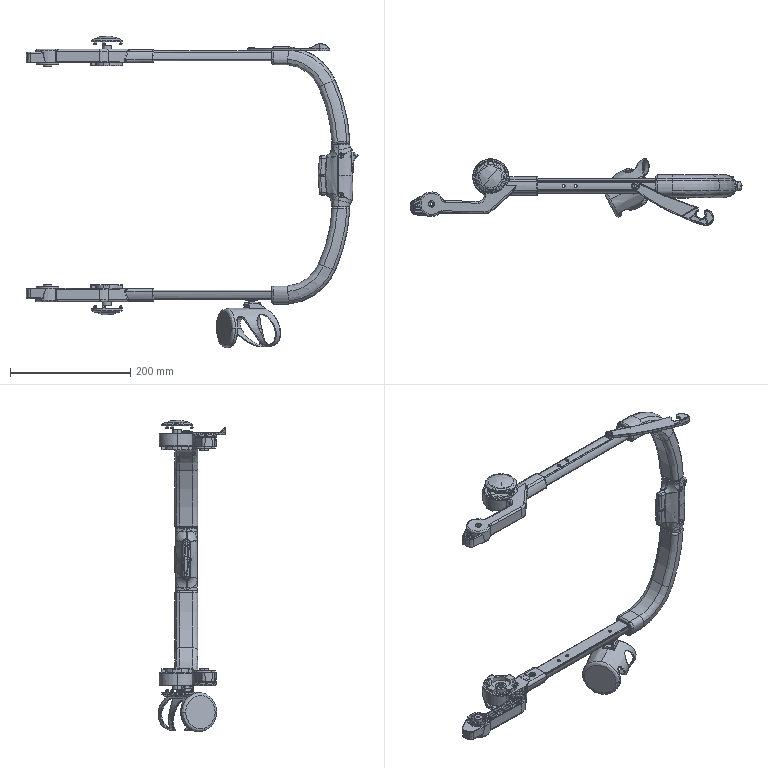Part | SolidWorks | 19 solids | 3815 faces | volume 680995 mm3 | spline 1394 | plane 1147 | cylinder 1052 | cone 120 | torus 60 | sphere 42 | commonest cylinder face diameters 1 x98 0.6 x65 2 x45 5.2 x42 1.003 x40 10 x37